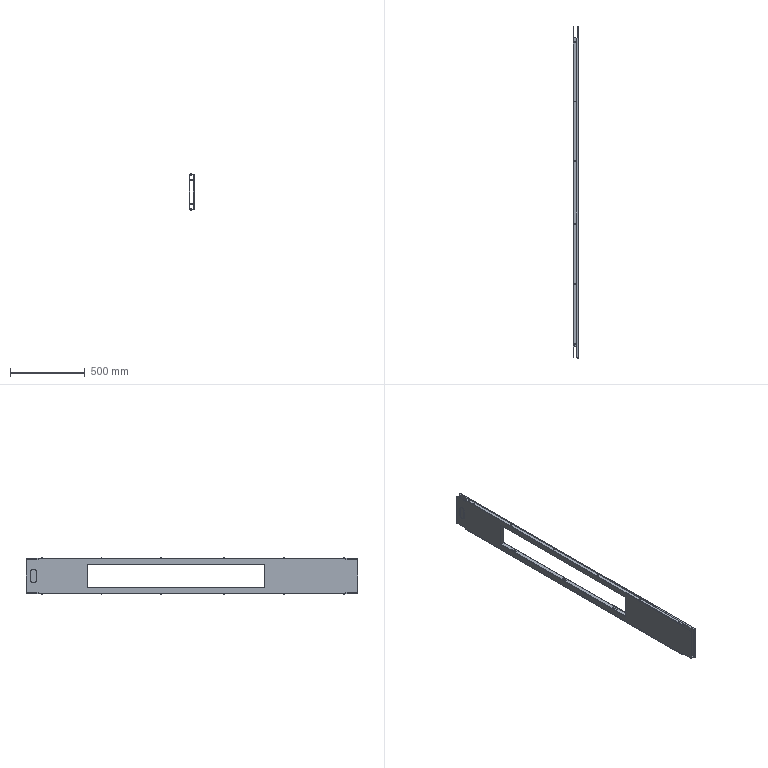Part | SolidWorks | features ReferencePattern 8, MirrorCompFeat 3 | 18 solids | 373 faces | box 36 x 2216 x 253 mm | volume 1444995 mm3 | plane 208 | cylinder 165 | commonest cylinder face diameters 8 x42 6 x32 6.2 x24 8.2 x24 12 x24 0.4 x6